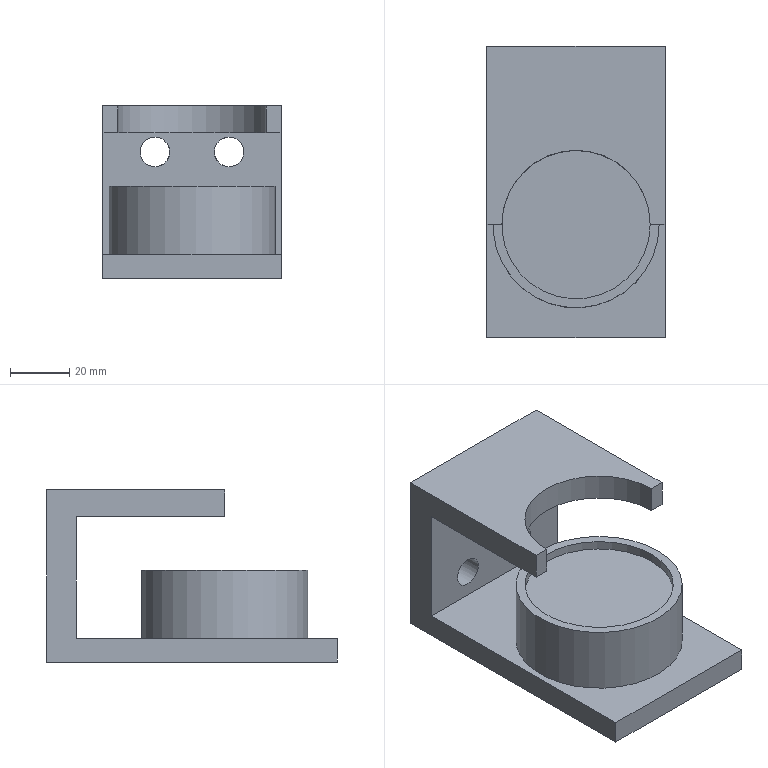Part | NX | features DATUM_CSYS 12, SKETCH 11, EXTRUDE 6, OFFSET_REGION 4, DATUM_PLANE 2, UNITE 1 | 1 solid | 20 faces | box 60 x 98 x 58 mm | volume 142821 mm3 | plane 13 | cylinder 7 | commonest cylinder face diameters 10 x4 50 x2 56 x1
STEP:
#1=CARTESIAN_POINT('',(88.,0.,13.));
#2=VERTEX_POINT('',#1);
#3=CARTESIAN_POINT('',(60.,0.,13.));
#4=DIRECTION('',(0.,0.,-1.));
#5=DIRECTION('',(1.,0.,0.));
#6=AXIS2_PLACEMENT_3D('',#3,#4,#5);
#7=CIRCLE('',#6,28.);
#8=EDGE_CURVE('',#2,#2,#7,.F.);
#9=ORIENTED_EDGE('',*,*,#8,.F.);
#10=EDGE_LOOP('',(#9));
#11=FACE_BOUND('',#10,.T.);
#12=CARTESIAN_POINT('',(88.,0.,-10.));
#13=VERTEX_POINT('',#12);
#14=CARTESIAN_POINT('',(60.,0.,-10.));
#15=DIRECTION('',(0.,0.,1.));
#16=DIRECTION('',(1.,0.,0.));
#17=AXIS2_PLACEMENT_3D('',#14,#15,#16);
#18=CIRCLE('',#17,28.);
#19=EDGE_CURVE('',#13,#13,#18,.F.);
#20=ORIENTED_EDGE('',*,*,#19,.F.);
#21=EDGE_LOOP('',(#20));
#22=FACE_BOUND('',#21,.T.);
#23=CARTESIAN_POINT('',(60.,0.,13.));
#24=DIRECTION('',(0.,0.,-1.));
#25=DIRECTION('',(-1.,0.,0.));
#26=AXIS2_PLACEMENT_3D('',#23,#24,#25);
#27=CYLINDRICAL_SURFACE('',#26,28.);
#28=ADVANCED_FACE('',(#11,#22),#27,.T.);
#29=CARTESIAN_POINT('',(85.,0.,13.));
#30=VERTEX_POINT('',#29);
#31=CARTESIAN_POINT('',(60.,0.,13.));
#32=DIRECTION('',(0.,0.,-1.));
#33=DIRECTION('',(1.,0.,0.));
#34=AXIS2_PLACEMENT_3D('',#31,#32,#33);
#35=CIRCLE('',#34,25.);
#36=EDGE_CURVE('',#30,#30,#35,.F.);
#37=ORIENTED_EDGE('',*,*,#36,.T.);
#38=EDGE_LOOP('',(#37));
#39=FACE_BOUND('',#38,.T.);
#40=CARTESIAN_POINT('',(85.,0.,10.));
#41=VERTEX_POINT('',#40);
#42=CARTESIAN_POINT('',(60.,0.,10.));
#43=DIRECTION('',(0.,0.,-1.));
#44=DIRECTION('',(1.,0.,0.));
#45=AXIS2_PLACEMENT_3D('',#42,#43,#44);
#46=CIRCLE('',#45,25.);
#47=EDGE_CURVE('',#41,#41,#46,.F.);
#48=ORIENTED_EDGE('',*,*,#47,.F.);
#49=EDGE_LOOP('',(#48));
#50=FACE_BOUND('',#49,.T.);
#51=CARTESIAN_POINT('',(60.,0.,13.));
#52=DIRECTION('',(0.,0.,-1.));
#53=DIRECTION('',(-1.,0.,0.));
#54=AXIS2_PLACEMENT_3D('',#51,#52,#53);
#55=CYLINDRICAL_SURFACE('',#54,25.);
#56=ADVANCED_FACE('',(#39,#50),#55,.F.);
#57=ORIENTED_EDGE('',*,*,#8,.T.);
#58=EDGE_LOOP('',(#57));
#59=FACE_BOUND('',#58,.T.);
#60=ORIENTED_EDGE('',*,*,#36,.F.);
#61=EDGE_LOOP('',(#60));
#62=FACE_BOUND('',#61,.T.);
#63=CARTESIAN_POINT('',(60.,0.,13.));
#64=DIRECTION('',(0.,0.,-1.));
#65=DIRECTION('',(-1.,0.,0.));
#66=AXIS2_PLACEMENT_3D('',#63,#64,#65);
#67=PLANE('',#66);
#68=ADVANCED_FACE('',(#59,#62),#67,.F.);
#69=ORIENTED_EDGE('',*,*,#47,.T.);
#70=EDGE_LOOP('',(#69));
#71=FACE_BOUND('',#70,.T.);
#72=CARTESIAN_POINT('',(60.,0.,10.));
#73=DIRECTION('',(0.,0.,-1.));
#74=DIRECTION('',(-1.,0.,0.));
#75=AXIS2_PLACEMENT_3D('',#72,#73,#74);
#76=PLANE('',#75);
#77=ADVANCED_FACE('',(#71),#76,.F.);
#78=CARTESIAN_POINT('',(85.,0.,40.));
#79=VERTEX_POINT('',#78);
#80=CARTESIAN_POINT('',(85.,0.,31.));
#81=VERTEX_POINT('',#80);
#82=CARTESIAN_POINT('',(85.,0.,30.));
#83=DIRECTION('',(0.,0.,1.));
#84=VECTOR('',#83,1000.);
#85=LINE('',#82,#84);
#86=EDGE_CURVE('',#79,#81,#85,.F.);
#87=ORIENTED_EDGE('',*,*,#86,.T.);
#88=CARTESIAN_POINT('',(90.,0.,31.));
#89=VERTEX_POINT('',#88);
#90=CARTESIAN_POINT('',(60.,0.,31.));
#91=DIRECTION('',(1.,0.,0.));
#92=VECTOR('',#91,1000.);
#93=LINE('',#90,#92);
#94=EDGE_CURVE('',#89,#81,#93,.F.);
#95=ORIENTED_EDGE('',*,*,#94,.F.);
#96=CARTESIAN_POINT('',(90.,0.,40.));
#97=VERTEX_POINT('',#96);
#98=CARTESIAN_POINT('',(90.,0.,30.));
#99=DIRECTION('',(0.,0.,1.));
#100=VECTOR('',#99,1000.);
#101=LINE('',#98,#100);
#102=EDGE_CURVE('',#97,#89,#101,.F.);
#103=ORIENTED_EDGE('',*,*,#102,.F.);
#104=CARTESIAN_POINT('',(85.,0.,40.));
#105=DIRECTION('',(-1.,0.,0.));
#106=VECTOR('',#105,1000.);
#107=LINE('',#104,#106);
#108=EDGE_CURVE('',#97,#79,#107,.T.);
#109=ORIENTED_EDGE('',*,*,#108,.T.);
#110=EDGE_LOOP('',(#87,#95,#103,#109));
#111=FACE_BOUND('',#110,.T.);
#112=CARTESIAN_POINT('',(85.,0.,35.));
#113=DIRECTION('',(0.,1.,0.));
#114=DIRECTION('',(0.,0.,1.));
#115=AXIS2_PLACEMENT_3D('',#112,#113,#114);
#116=PLANE('',#115);
#117=ADVANCED_FACE('',(#111),#116,.F.);
#118=CARTESIAN_POINT('',(35.,0.,40.));
#119=VERTEX_POINT('',#118);
#120=CARTESIAN_POINT('',(35.,0.,31.));
#121=VERTEX_POINT('',#120);
#122=CARTESIAN_POINT('',(35.,0.,30.));
#123=DIRECTION('',(0.,0.,1.));
#124=VECTOR('',#123,1000.);
#125=LINE('',#122,#124);
#126=EDGE_CURVE('',#119,#121,#125,.F.);
#127=ORIENTED_EDGE('',*,*,#126,.F.);
#128=CARTESIAN_POINT('',(30.,0.,40.));
#129=VERTEX_POINT('',#128);
#130=CARTESIAN_POINT('',(35.,0.,40.));
#131=DIRECTION('',(1.,0.,0.));
#132=VECTOR('',#131,1000.);
#133=LINE('',#130,#132);
#134=EDGE_CURVE('',#129,#119,#133,.T.);
#135=ORIENTED_EDGE('',*,*,#134,.F.);
#136=CARTESIAN_POINT('',(30.,0.,31.));
#137=VERTEX_POINT('',#136);
#138=CARTESIAN_POINT('',(30.,0.,35.));
#139=DIRECTION('',(0.,0.,-1.));
#140=VECTOR('',#139,1000.);
#141=LINE('',#138,#140);
#142=EDGE_CURVE('',#129,#137,#141,.T.);
#143=ORIENTED_EDGE('',*,*,#142,.T.);
#144=CARTESIAN_POINT('',(35.,0.,31.));
#145=DIRECTION('',(1.,0.,0.));
#146=VECTOR('',#145,1000.);
#147=LINE('',#144,#146);
#148=EDGE_CURVE('',#137,#121,#147,.T.);
#149=ORIENTED_EDGE('',*,*,#148,.T.);
#150=EDGE_LOOP('',(#127,#135,#143,#149));
#151=FACE_BOUND('',#150,.T.);
#152=CARTESIAN_POINT('',(35.,0.,35.));
#153=DIRECTION('',(0.,-1.,0.));
#154=DIRECTION('',(0.,0.,1.));
#155=AXIS2_PLACEMENT_3D('',#152,#153,#154);
#156=PLANE('',#155);
#157=ADVANCED_FACE('',(#151),#156,.T.);
#158=CARTESIAN_POINT('',(30.,50.,31.));
#159=VERTEX_POINT('',#158);
#160=CARTESIAN_POINT('',(30.,0.,31.));
#161=DIRECTION('',(0.,1.,0.));
#162=VECTOR('',#161,1000.);
#163=LINE('',#160,#162);
#164=EDGE_CURVE('',#137,#159,#163,.T.);
#165=ORIENTED_EDGE('',*,*,#164,.T.);
#166=CARTESIAN_POINT('',(90.,50.,31.));
#167=VERTEX_POINT('',#166);
#168=CARTESIAN_POINT('',(60.,50.,31.));
#169=DIRECTION('',(1.,0.,0.));
#170=VECTOR('',#169,1000.);
#171=LINE('',#168,#170);
#172=EDGE_CURVE('',#159,#167,#171,.T.);
#173=ORIENTED_EDGE('',*,*,#172,.T.);
#174=CARTESIAN_POINT('',(90.,0.,31.));
#175=DIRECTION('',(0.,-1.,0.));
#176=VECTOR('',#175,1000.);
#177=LINE('',#174,#176);
#178=EDGE_CURVE('',#167,#89,#177,.T.);
#179=ORIENTED_EDGE('',*,*,#178,.T.);
#180=ORIENTED_EDGE('',*,*,#94,.T.);
#181=CARTESIAN_POINT('',(60.,0.,31.));
#182=DIRECTION('',(0.,0.,-1.));
#183=DIRECTION('',(-1.,0.,0.));
#184=AXIS2_PLACEMENT_3D('',#181,#182,#183);
#185=CIRCLE('',#184,25.);
#186=EDGE_CURVE('',#81,#121,#185,.F.);
#187=ORIENTED_EDGE('',*,*,#186,.T.);
#188=ORIENTED_EDGE('',*,*,#148,.F.);
#189=EDGE_LOOP('',(#165,#173,#179,#180,#187,#188));
#190=FACE_BOUND('',#189,.T.);
#191=CARTESIAN_POINT('',(60.,0.,31.));
#192=DIRECTION('',(0.,0.,-1.));
#193=DIRECTION('',(-1.,0.,0.));
#194=AXIS2_PLACEMENT_3D('',#191,#192,#193);
#195=PLANE('',#194);
#196=ADVANCED_FACE('',(#190),#195,.T.);
#197=CARTESIAN_POINT('',(30.,-38.,-18.));
#198=VERTEX_POINT('',#197);
#199=CARTESIAN_POINT('',(30.,60.,-18.));
#200=VERTEX_POINT('',#199);
#201=CARTESIAN_POINT('',(30.,50.,-18.));
#202=DIRECTION('',(0.,1.,0.));
#203=VECTOR('',#202,1000.);
#204=LINE('',#201,#203);
#205=EDGE_CURVE('',#198,#200,#204,.T.);
#206=ORIENTED_EDGE('',*,*,#205,.F.);
#207=CARTESIAN_POINT('',(30.,-38.,-10.));
#208=VERTEX_POINT('',#207);
#209=CARTESIAN_POINT('',(30.,-38.,30.));
#210=DIRECTION('',(0.,0.,-1.));
#211=VECTOR('',#210,1000.);
#212=LINE('',#209,#211);
#213=EDGE_CURVE('',#208,#198,#212,.T.);
#214=ORIENTED_EDGE('',*,*,#213,.F.);
#215=CARTESIAN_POINT('',(30.,50.,-10.));
#216=VERTEX_POINT('',#215);
#217=CARTESIAN_POINT('',(30.,60.,-10.));
#218=DIRECTION('',(0.,-1.,0.));
#219=VECTOR('',#218,1000.);
#220=LINE('',#217,#219);
#221=EDGE_CURVE('',#216,#208,#220,.T.);
#222=ORIENTED_EDGE('',*,*,#221,.F.);
#223=CARTESIAN_POINT('',(30.,50.,0.));
#224=DIRECTION('',(0.,0.,1.));
#225=VECTOR('',#224,1000.);
#226=LINE('',#223,#225);
#227=EDGE_CURVE('',#216,#159,#226,.T.);
#228=ORIENTED_EDGE('',*,*,#227,.T.);
#229=ORIENTED_EDGE('',*,*,#164,.F.);
#230=ORIENTED_EDGE('',*,*,#142,.F.);
#231=CARTESIAN_POINT('',(30.,60.,40.));
#232=VERTEX_POINT('',#231);
#233=CARTESIAN_POINT('',(30.,0.,40.));
#234=DIRECTION('',(0.,1.,0.));
#235=VECTOR('',#234,1000.);
#236=LINE('',#233,#235);
#237=EDGE_CURVE('',#129,#232,#236,.T.);
#238=ORIENTED_EDGE('',*,*,#237,.T.);
#239=CARTESIAN_POINT('',(30.,60.,30.));
#240=DIRECTION('',(0.,0.,-1.));
#241=VECTOR('',#240,1000.);
#242=LINE('',#239,#241);
#243=EDGE_CURVE('',#232,#200,#242,.T.);
#244=ORIENTED_EDGE('',*,*,#243,.T.);
#245=EDGE_LOOP('',(#206,#214,#222,#228,#229,#230,#238,#244));
#246=FACE_BOUND('',#245,.T.);
#247=CARTESIAN_POINT('',(30.,60.,30.));
#248=DIRECTION('',(-1.,0.,0.));
#249=DIRECTION('',(0.,-1.,0.));
#250=AXIS2_PLACEMENT_3D('',#247,#248,#249);
#251=PLANE('',#250);
#252=ADVANCED_FACE('',(#246),#251,.T.);
#253=CARTESIAN_POINT('',(60.,0.,40.));
#254=DIRECTION('',(0.,0.,-1.));
#255=DIRECTION('',(1.,0.,0.));
#256=AXIS2_PLACEMENT_3D('',#253,#254,#255);
#257=CIRCLE('',#256,25.);
#258=EDGE_CURVE('',#79,#119,#257,.F.);
#259=ORIENTED_EDGE('',*,*,#258,.T.);
#260=ORIENTED_EDGE('',*,*,#126,.T.);
#261=ORIENTED_EDGE('',*,*,#186,.F.);
#262=ORIENTED_EDGE('',*,*,#86,.F.);
#263=EDGE_LOOP('',(#259,#260,#261,#262));
#264=FACE_BOUND('',#263,.T.);
#265=CARTESIAN_POINT('',(60.,0.,30.));
#266=DIRECTION('',(0.,0.,1.));
#267=DIRECTION('',(1.,0.,0.));
#268=AXIS2_PLACEMENT_3D('',#265,#266,#267);
#269=CYLINDRICAL_SURFACE('',#268,25.);
#270=ADVANCED_FACE('',(#264),#269,.F.);
#271=CARTESIAN_POINT('',(90.,-38.,-18.));
#272=VERTEX_POINT('',#271);
#273=CARTESIAN_POINT('',(90.,60.,-18.));
#274=VERTEX_POINT('',#273);
#275=CARTESIAN_POINT('',(90.,0.,-18.));
#276=DIRECTION('',(0.,1.,0.));
#277=VECTOR('',#276,1000.);
#278=LINE('',#275,#277);
#279=EDGE_CURVE('',#272,#274,#278,.T.);
#280=ORIENTED_EDGE('',*,*,#279,.T.);
#281=CARTESIAN_POINT('',(90.,60.,40.));
#282=VERTEX_POINT('',#281);
#283=CARTESIAN_POINT('',(90.,60.,30.));
#284=DIRECTION('',(0.,0.,-1.));
#285=VECTOR('',#284,1000.);
#286=LINE('',#283,#285);
#287=EDGE_CURVE('',#282,#274,#286,.T.);
#288=ORIENTED_EDGE('',*,*,#287,.F.);
#289=CARTESIAN_POINT('',(90.,0.,40.));
#290=DIRECTION('',(0.,-1.,0.));
#291=VECTOR('',#290,1000.);
#292=LINE('',#289,#291);
#293=EDGE_CURVE('',#282,#97,#292,.T.);
#294=ORIENTED_EDGE('',*,*,#293,.T.);
#295=ORIENTED_EDGE('',*,*,#102,.T.);
#296=ORIENTED_EDGE('',*,*,#178,.F.);
#297=CARTESIAN_POINT('',(90.,50.,-10.));
#298=VERTEX_POINT('',#297);
#299=CARTESIAN_POINT('',(90.,50.,0.));
#300=DIRECTION('',(0.,0.,-1.));
#301=VECTOR('',#300,1000.);
#302=LINE('',#299,#301);
#303=EDGE_CURVE('',#167,#298,#302,.T.);
#304=ORIENTED_EDGE('',*,*,#303,.T.);
#305=CARTESIAN_POINT('',(90.,-38.,-10.));
#306=VERTEX_POINT('',#305);
#307=CARTESIAN_POINT('',(90.,-30.,-10.));
#308=DIRECTION('',(0.,1.,0.));
#309=VECTOR('',#308,1000.);
#310=LINE('',#307,#309);
#311=EDGE_CURVE('',#306,#298,#310,.T.);
#312=ORIENTED_EDGE('',*,*,#311,.F.);
#313=CARTESIAN_POINT('',(90.,-38.,-10.));
#314=DIRECTION('',(0.,0.,-1.));
#315=VECTOR('',#314,1000.);
#316=LINE('',#313,#315);
#317=EDGE_CURVE('',#306,#272,#316,.T.);
#318=ORIENTED_EDGE('',*,*,#317,.T.);
#319=EDGE_LOOP('',(#280,#288,#294,#295,#296,#304,#312,#318));
#320=FACE_BOUND('',#319,.T.);
#321=CARTESIAN_POINT('',(90.,0.,30.));
#322=DIRECTION('',(1.,0.,0.));
#323=DIRECTION('',(0.,1.,0.));
#324=AXIS2_PLACEMENT_3D('',#321,#322,#323);
#325=PLANE('',#324);
#326=ADVANCED_FACE('',(#320),#325,.T.);
#327=CARTESIAN_POINT('',(67.5,60.,-0.5));
#328=VERTEX_POINT('',#327);
#329=CARTESIAN_POINT('',(72.5,60.,-0.5));
#330=DIRECTION('',(0.,1.,0.));
#331=DIRECTION('',(-1.,0.,0.));
#332=AXIS2_PLACEMENT_3D('',#329,#330,#331);
#333=CIRCLE('',#332,5.);
#334=EDGE_CURVE('',#328,#328,#333,.T.);
#335=ORIENTED_EDGE('',*,*,#334,.F.);
#336=EDGE_LOOP('',(#335));
#337=FACE_BOUND('',#336,.T.);
#338=CARTESIAN_POINT('',(42.5,60.,24.5));
#339=VERTEX_POINT('',#338);
#340=CARTESIAN_POINT('',(47.5,60.,24.5));
#341=DIRECTION('',(0.,1.,0.));
#342=DIRECTION('',(-1.,0.,0.));
#343=AXIS2_PLACEMENT_3D('',#340,#341,#342);
#344=CIRCLE('',#343,5.);
#345=EDGE_CURVE('',#339,#339,#344,.T.);
#346=ORIENTED_EDGE('',*,*,#345,.F.);
#347=EDGE_LOOP('',(#346));
#348=FACE_BOUND('',#347,.T.);
#349=CARTESIAN_POINT('',(42.5,60.,-0.5));
#350=VERTEX_POINT('',#349);
#351=CARTESIAN_POINT('',(47.5,60.,-0.5));
#352=DIRECTION('',(0.,1.,0.));
#353=DIRECTION('',(-1.,0.,0.));
#354=AXIS2_PLACEMENT_3D('',#351,#352,#353);
#355=CIRCLE('',#354,5.);
#356=EDGE_CURVE('',#350,#350,#355,.T.);
#357=ORIENTED_EDGE('',*,*,#356,.F.);
#358=EDGE_LOOP('',(#357));
#359=FACE_BOUND('',#358,.T.);
#360=CARTESIAN_POINT('',(67.5,60.,24.5));
#361=VERTEX_POINT('',#360);
#362=CARTESIAN_POINT('',(72.5,60.,24.5));
#363=DIRECTION('',(0.,1.,0.));
#364=DIRECTION('',(-1.,0.,0.));
#365=AXIS2_PLACEMENT_3D('',#362,#363,#364);
#366=CIRCLE('',#365,5.);
#367=EDGE_CURVE('',#361,#361,#366,.T.);
#368=ORIENTED_EDGE('',*,*,#367,.F.);
#369=EDGE_LOOP('',(#368));
#370=FACE_BOUND('',#369,.T.);
#371=CARTESIAN_POINT('',(85.,60.,-18.));
#372=DIRECTION('',(-1.,0.,0.));
#373=VECTOR('',#372,1000.);
#374=LINE('',#371,#373);
#375=EDGE_CURVE('',#274,#200,#374,.T.);
#376=ORIENTED_EDGE('',*,*,#375,.T.);
#377=ORIENTED_EDGE('',*,*,#243,.F.);
#378=CARTESIAN_POINT('',(85.,60.,40.));
#379=DIRECTION('',(-1.,0.,0.));
#380=VECTOR('',#379,1000.);
#381=LINE('',#378,#380);
#382=EDGE_CURVE('',#232,#282,#381,.F.);
#383=ORIENTED_EDGE('',*,*,#382,.T.);
#384=ORIENTED_EDGE('',*,*,#287,.T.);
#385=EDGE_LOOP('',(#376,#377,#383,#384));
#386=FACE_BOUND('',#385,.T.);
#387=CARTESIAN_POINT('',(85.,60.,30.));
#388=DIRECTION('',(0.,1.,0.));
#389=DIRECTION('',(0.,0.,1.));
#390=AXIS2_PLACEMENT_3D('',#387,#388,#389);
#391=PLANE('',#390);
#392=ADVANCED_FACE('',(#337,#348,#359,#370,#386),#391,.T.);
#393=ORIENTED_EDGE('',*,*,#382,.F.);
#394=ORIENTED_EDGE('',*,*,#237,.F.);
#395=ORIENTED_EDGE('',*,*,#134,.T.);
#396=ORIENTED_EDGE('',*,*,#258,.F.);
#397=ORIENTED_EDGE('',*,*,#108,.F.);
#398=ORIENTED_EDGE('',*,*,#293,.F.);
#399=EDGE_LOOP('',(#393,#394,#395,#396,#397,#398));
#400=FACE_BOUND('',#399,.T.);
#401=CARTESIAN_POINT('',(60.,0.,40.));
#402=DIRECTION('',(0.,0.,-1.));
#403=DIRECTION('',(-1.,0.,0.));
#404=AXIS2_PLACEMENT_3D('',#401,#402,#403);
#405=PLANE('',#404);
#406=ADVANCED_FACE('',(#400),#405,.F.);
#407=ORIENTED_EDGE('',*,*,#375,.F.);
#408=ORIENTED_EDGE('',*,*,#279,.F.);
#409=CARTESIAN_POINT('',(85.,-38.,-18.));
#410=DIRECTION('',(1.,0.,0.));
#411=VECTOR('',#410,1000.);
#412=LINE('',#409,#411);
#413=EDGE_CURVE('',#198,#272,#412,.T.);
#414=ORIENTED_EDGE('',*,*,#413,.F.);
#415=ORIENTED_EDGE('',*,*,#205,.T.);
#416=EDGE_LOOP('',(#407,#408,#414,#415));
#417=FACE_BOUND('',#416,.T.);
#418=CARTESIAN_POINT('',(85.,50.,-18.));
#419=DIRECTION('',(0.,0.,-1.));
#420=DIRECTION('',(-1.,0.,0.));
#421=AXIS2_PLACEMENT_3D('',#418,#419,#420);
#422=PLANE('',#421);
#423=ADVANCED_FACE('',(#417),#422,.T.);
#424=CARTESIAN_POINT('',(72.5,50.,4.5));
#425=VERTEX_POINT('',#424);
#426=CARTESIAN_POINT('',(72.5,50.,-0.5));
#427=DIRECTION('',(0.,1.,0.));
#428=DIRECTION('',(0.,0.,1.));
#429=AXIS2_PLACEMENT_3D('',#426,#427,#428);
#430=CIRCLE('',#429,5.);
#431=EDGE_CURVE('',#425,#425,#430,.T.);
#432=ORIENTED_EDGE('',*,*,#431,.T.);
#433=EDGE_LOOP('',(#432));
#434=FACE_BOUND('',#433,.T.);
#435=CARTESIAN_POINT('',(47.5,50.,29.5));
#436=VERTEX_POINT('',#435);
#437=CARTESIAN_POINT('',(47.5,50.,24.5));
#438=DIRECTION('',(0.,1.,0.));
#439=DIRECTION('',(0.,0.,1.));
#440=AXIS2_PLACEMENT_3D('',#437,#438,#439);
#441=CIRCLE('',#440,5.);
#442=EDGE_CURVE('',#436,#436,#441,.T.);
#443=ORIENTED_EDGE('',*,*,#442,.T.);
#444=EDGE_LOOP('',(#443));
#445=FACE_BOUND('',#444,.T.);
#446=CARTESIAN_POINT('',(47.5,50.,4.5));
#447=VERTEX_POINT('',#446);
#448=CARTESIAN_POINT('',(47.5,50.,-0.5));
#449=DIRECTION('',(0.,1.,0.));
#450=DIRECTION('',(0.,0.,1.));
#451=AXIS2_PLACEMENT_3D('',#448,#449,#450);
#452=CIRCLE('',#451,5.);
#453=EDGE_CURVE('',#447,#447,#452,.T.);
#454=ORIENTED_EDGE('',*,*,#453,.T.);
#455=EDGE_LOOP('',(#454));
#456=FACE_BOUND('',#455,.T.);
#457=CARTESIAN_POINT('',(72.5,50.,29.5));
#458=VERTEX_POINT('',#457);
#459=CARTESIAN_POINT('',(72.5,50.,24.5));
#460=DIRECTION('',(0.,1.,0.));
#461=DIRECTION('',(0.,0.,1.));
#462=AXIS2_PLACEMENT_3D('',#459,#460,#461);
#463=CIRCLE('',#462,5.);
#464=EDGE_CURVE('',#458,#458,#463,.T.);
#465=ORIENTED_EDGE('',*,*,#464,.T.);
#466=EDGE_LOOP('',(#465));
#467=FACE_BOUND('',#466,.T.);
#468=ORIENTED_EDGE('',*,*,#227,.F.);
#469=CARTESIAN_POINT('',(0.,50.,-10.));
#470=DIRECTION('',(1.,0.,0.));
#471=VECTOR('',#470,1000.);
#472=LINE('',#469,#471);
#473=EDGE_CURVE('',#216,#298,#472,.T.);
#474=ORIENTED_EDGE('',*,*,#473,.T.);
#475=ORIENTED_EDGE('',*,*,#303,.F.);
#476=ORIENTED_EDGE('',*,*,#172,.F.);
#477=EDGE_LOOP('',(#468,#474,#475,#476));
#478=FACE_BOUND('',#477,.T.);
#479=CARTESIAN_POINT('',(0.,50.,0.));
#480=DIRECTION('',(0.,1.,0.));
#481=DIRECTION('',(0.,0.,1.));
#482=AXIS2_PLACEMENT_3D('',#479,#480,#481);
#483=PLANE('',#482);
#484=ADVANCED_FACE('',(#434,#445,#456,#467,#478),#483,.F.);
#485=ORIENTED_EDGE('',*,*,#19,.T.);
#486=EDGE_LOOP('',(#485));
#487=FACE_BOUND('',#486,.T.);
#488=ORIENTED_EDGE('',*,*,#473,.F.);
#489=ORIENTED_EDGE('',*,*,#221,.T.);
#490=CARTESIAN_POINT('',(30.,-38.,-10.));
#491=DIRECTION('',(1.,0.,0.));
#492=VECTOR('',#491,1000.);
#493=LINE('',#490,#492);
#494=EDGE_CURVE('',#208,#306,#493,.T.);
#495=ORIENTED_EDGE('',*,*,#494,.T.);
#496=ORIENTED_EDGE('',*,*,#311,.T.);
#497=EDGE_LOOP('',(#488,#489,#495,#496));
#498=FACE_BOUND('',#497,.T.);
#499=CARTESIAN_POINT('',(0.,0.,-10.));
#500=DIRECTION('',(0.,0.,1.));
#501=DIRECTION('',(1.,0.,0.));
#502=AXIS2_PLACEMENT_3D('',#499,#500,#501);
#503=PLANE('',#502);
#504=ADVANCED_FACE('',(#487,#498),#503,.T.);
#505=ORIENTED_EDGE('',*,*,#413,.T.);
#506=ORIENTED_EDGE('',*,*,#317,.F.);
#507=ORIENTED_EDGE('',*,*,#494,.F.);
#508=ORIENTED_EDGE('',*,*,#213,.T.);
#509=EDGE_LOOP('',(#505,#506,#507,#508));
#510=FACE_BOUND('',#509,.T.);
#511=CARTESIAN_POINT('',(30.,-38.,-10.));
#512=DIRECTION('',(0.,1.,0.));
#513=DIRECTION('',(-1.,0.,0.));
#514=AXIS2_PLACEMENT_3D('',#511,#512,#513);
#515=PLANE('',#514);
#516=ADVANCED_FACE('',(#510),#515,.F.);
#517=ORIENTED_EDGE('',*,*,#367,.T.);
#518=EDGE_LOOP('',(#517));
#519=FACE_BOUND('',#518,.T.);
#520=ORIENTED_EDGE('',*,*,#464,.F.);
#521=EDGE_LOOP('',(#520));
#522=FACE_BOUND('',#521,.T.);
#523=CARTESIAN_POINT('',(72.5,30.,24.5));
#524=DIRECTION('',(0.,1.,0.));
#525=DIRECTION('',(0.,0.,1.));
#526=AXIS2_PLACEMENT_3D('',#523,#524,#525);
#527=CYLINDRICAL_SURFACE('',#526,5.);
#528=ADVANCED_FACE('',(#519,#522),#527,.F.);
#529=ORIENTED_EDGE('',*,*,#356,.T.);
#530=EDGE_LOOP('',(#529));
#531=FACE_BOUND('',#530,.T.);
#532=ORIENTED_EDGE('',*,*,#453,.F.);
#533=EDGE_LOOP('',(#532));
#534=FACE_BOUND('',#533,.T.);
#535=CARTESIAN_POINT('',(47.5,30.,-0.5));
#536=DIRECTION('',(0.,1.,0.));
#537=DIRECTION('',(0.,0.,1.));
#538=AXIS2_PLACEMENT_3D('',#535,#536,#537);
#539=CYLINDRICAL_SURFACE('',#538,5.);
#540=ADVANCED_FACE('',(#531,#534),#539,.F.);
#541=ORIENTED_EDGE('',*,*,#345,.T.);
#542=EDGE_LOOP('',(#541));
#543=FACE_BOUND('',#542,.T.);
#544=ORIENTED_EDGE('',*,*,#442,.F.);
#545=EDGE_LOOP('',(#544));
#546=FACE_BOUND('',#545,.T.);
#547=CARTESIAN_POINT('',(47.5,30.,24.5));
#548=DIRECTION('',(0.,1.,0.));
#549=DIRECTION('',(0.,0.,1.));
#550=AXIS2_PLACEMENT_3D('',#547,#548,#549);
#551=CYLINDRICAL_SURFACE('',#550,5.);
#552=ADVANCED_FACE('',(#543,#546),#551,.F.);
#553=ORIENTED_EDGE('',*,*,#334,.T.);
#554=EDGE_LOOP('',(#553));
#555=FACE_BOUND('',#554,.T.);
#556=ORIENTED_EDGE('',*,*,#431,.F.);
#557=EDGE_LOOP('',(#556));
#558=FACE_BOUND('',#557,.T.);
#559=CARTESIAN_POINT('',(72.5,30.,-0.5));
#560=DIRECTION('',(0.,1.,0.));
#561=DIRECTION('',(0.,0.,1.));
#562=AXIS2_PLACEMENT_3D('',#559,#560,#561);
#563=CYLINDRICAL_SURFACE('',#562,5.);
#564=ADVANCED_FACE('',(#555,#558),#563,.F.);
#565=CLOSED_SHELL('',(#28,#56,#68,#77,#117,#157,#196,#252,#270,#326,#392,#406,#423,#484,#504,#516,#528,#540,#552,#564));
#566=MANIFOLD_SOLID_BREP('',#565);
#567=(LENGTH_UNIT()NAMED_UNIT(*)SI_UNIT(.MILLI.,.METRE.));
#568=UNCERTAINTY_MEASURE_WITH_UNIT(LENGTH_MEASURE(0.00001),#567,'','');
#569=(NAMED_UNIT(*)PLANE_ANGLE_UNIT()SI_UNIT($,.RADIAN.));
#570=(NAMED_UNIT(*)SI_UNIT($,.STERADIAN.)SOLID_ANGLE_UNIT());
#571=(GEOMETRIC_REPRESENTATION_CONTEXT(3)GLOBAL_UNCERTAINTY_ASSIGNED_CONTEXT((#568))GLOBAL_UNIT_ASSIGNED_CONTEXT((#567,#569,#570))REPRESENTATION_CONTEXT('',''));
#572=ADVANCED_BREP_SHAPE_REPRESENTATION('',(#566),#571);